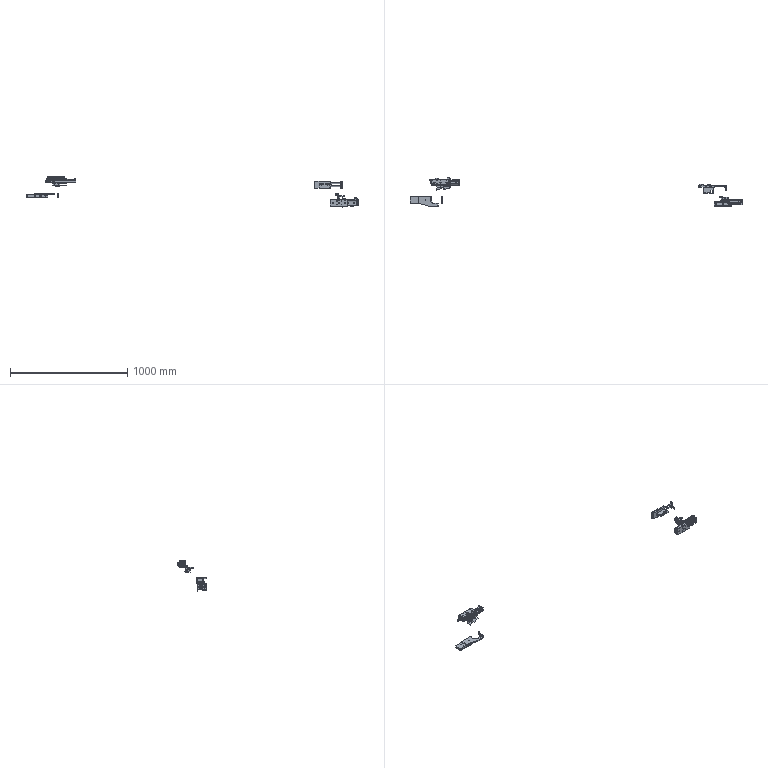Part | NX | 46 solids | 2799 faces | box 2831 x 244 x 259 mm | volume 1566156 mm3 | plane 1420 | cylinder 1039 | cone 340 | commonest cylinder face diameters 5 x229 4 x124 2.5 x94 10 x42 5.5 x41 6 x40